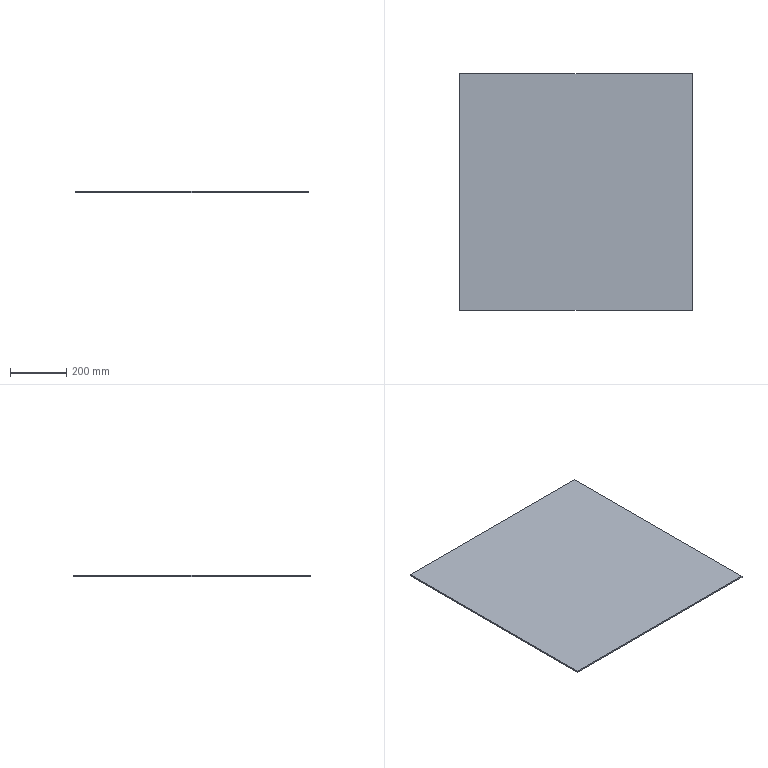Part | SolidWorks | features Extrusion 1, HoleWzd 1 | 1 solid | 6 faces | box 829 x 842 x 5 mm | volume 3490090 mm3 | plane 6
STEP:
#1=CARTESIAN_POINT('',(414.5,-421.,0.));
#2=VERTEX_POINT('',#1);
#3=CARTESIAN_POINT('',(414.5,421.,0.));
#4=VERTEX_POINT('',#3);
#5=CARTESIAN_POINT('',(414.5,421.,0.));
#6=DIRECTION('',(0.,1.,0.));
#7=VECTOR('',#6,1000.);
#8=LINE('',#5,#7);
#9=EDGE_CURVE('',#2,#4,#8,.T.);
#10=ORIENTED_EDGE('',*,*,#9,.T.);
#11=CARTESIAN_POINT('',(414.5,421.,5.));
#12=VERTEX_POINT('',#11);
#13=CARTESIAN_POINT('',(414.5,421.,5.));
#14=DIRECTION('',(0.,0.,-1.));
#15=VECTOR('',#14,1000.);
#16=LINE('',#13,#15);
#17=EDGE_CURVE('',#12,#4,#16,.T.);
#18=ORIENTED_EDGE('',*,*,#17,.F.);
#19=CARTESIAN_POINT('',(414.5,-421.,5.));
#20=VERTEX_POINT('',#19);
#21=CARTESIAN_POINT('',(414.5,421.,5.));
#22=DIRECTION('',(0.,1.,0.));
#23=VECTOR('',#22,1000.);
#24=LINE('',#21,#23);
#25=EDGE_CURVE('',#20,#12,#24,.T.);
#26=ORIENTED_EDGE('',*,*,#25,.F.);
#27=CARTESIAN_POINT('',(414.5,-421.,5.));
#28=DIRECTION('',(0.,0.,-1.));
#29=VECTOR('',#28,1000.);
#30=LINE('',#27,#29);
#31=EDGE_CURVE('',#20,#2,#30,.T.);
#32=ORIENTED_EDGE('',*,*,#31,.T.);
#33=EDGE_LOOP('',(#10,#18,#26,#32));
#34=FACE_OUTER_BOUND('',#33,.T.);
#35=CARTESIAN_POINT('',(414.5,421.,5.));
#36=DIRECTION('',(-1.,0.,0.));
#37=DIRECTION('',(0.,-1.,0.));
#38=AXIS2_PLACEMENT_3D('',#35,#36,#37);
#39=PLANE('',#38);
#40=ADVANCED_FACE('',(#34),#39,.F.);
#41=CARTESIAN_POINT('',(-414.5,421.,0.));
#42=VERTEX_POINT('',#41);
#43=CARTESIAN_POINT('',(-414.5,421.,0.));
#44=DIRECTION('',(-1.,0.,0.));
#45=VECTOR('',#44,1000.);
#46=LINE('',#43,#45);
#47=EDGE_CURVE('',#4,#42,#46,.T.);
#48=ORIENTED_EDGE('',*,*,#47,.T.);
#49=CARTESIAN_POINT('',(-414.5,421.,5.));
#50=VERTEX_POINT('',#49);
#51=CARTESIAN_POINT('',(-414.5,421.,5.));
#52=DIRECTION('',(0.,0.,-1.));
#53=VECTOR('',#52,1000.);
#54=LINE('',#51,#53);
#55=EDGE_CURVE('',#50,#42,#54,.T.);
#56=ORIENTED_EDGE('',*,*,#55,.F.);
#57=CARTESIAN_POINT('',(-414.5,421.,5.));
#58=DIRECTION('',(-1.,0.,0.));
#59=VECTOR('',#58,1000.);
#60=LINE('',#57,#59);
#61=EDGE_CURVE('',#12,#50,#60,.T.);
#62=ORIENTED_EDGE('',*,*,#61,.F.);
#63=ORIENTED_EDGE('',*,*,#17,.T.);
#64=EDGE_LOOP('',(#48,#56,#62,#63));
#65=FACE_OUTER_BOUND('',#64,.T.);
#66=CARTESIAN_POINT('',(-414.5,421.,5.));
#67=DIRECTION('',(0.,-1.,0.));
#68=DIRECTION('',(0.,0.,-1.));
#69=AXIS2_PLACEMENT_3D('',#66,#67,#68);
#70=PLANE('',#69);
#71=ADVANCED_FACE('',(#65),#70,.F.);
#72=CARTESIAN_POINT('',(-414.5,-421.,0.));
#73=VERTEX_POINT('',#72);
#74=CARTESIAN_POINT('',(-414.5,421.,0.));
#75=DIRECTION('',(0.,-1.,0.));
#76=VECTOR('',#75,1000.);
#77=LINE('',#74,#76);
#78=EDGE_CURVE('',#42,#73,#77,.T.);
#79=ORIENTED_EDGE('',*,*,#78,.T.);
#80=CARTESIAN_POINT('',(-414.5,-421.,5.));
#81=VERTEX_POINT('',#80);
#82=CARTESIAN_POINT('',(-414.5,-421.,5.));
#83=DIRECTION('',(0.,0.,-1.));
#84=VECTOR('',#83,1000.);
#85=LINE('',#82,#84);
#86=EDGE_CURVE('',#81,#73,#85,.T.);
#87=ORIENTED_EDGE('',*,*,#86,.F.);
#88=CARTESIAN_POINT('',(-414.5,421.,5.));
#89=DIRECTION('',(0.,-1.,0.));
#90=VECTOR('',#89,1000.);
#91=LINE('',#88,#90);
#92=EDGE_CURVE('',#50,#81,#91,.T.);
#93=ORIENTED_EDGE('',*,*,#92,.F.);
#94=ORIENTED_EDGE('',*,*,#55,.T.);
#95=EDGE_LOOP('',(#79,#87,#93,#94));
#96=FACE_OUTER_BOUND('',#95,.T.);
#97=CARTESIAN_POINT('',(-414.5,421.,5.));
#98=DIRECTION('',(1.,0.,0.));
#99=DIRECTION('',(0.,1.,0.));
#100=AXIS2_PLACEMENT_3D('',#97,#98,#99);
#101=PLANE('',#100);
#102=ADVANCED_FACE('',(#96),#101,.F.);
#103=CARTESIAN_POINT('',(-414.5,-421.,0.));
#104=DIRECTION('',(1.,0.,0.));
#105=VECTOR('',#104,1000.);
#106=LINE('',#103,#105);
#107=EDGE_CURVE('',#73,#2,#106,.T.);
#108=ORIENTED_EDGE('',*,*,#107,.T.);
#109=ORIENTED_EDGE('',*,*,#31,.F.);
#110=CARTESIAN_POINT('',(-414.5,-421.,5.));
#111=DIRECTION('',(1.,0.,0.));
#112=VECTOR('',#111,1000.);
#113=LINE('',#110,#112);
#114=EDGE_CURVE('',#81,#20,#113,.T.);
#115=ORIENTED_EDGE('',*,*,#114,.F.);
#116=ORIENTED_EDGE('',*,*,#86,.T.);
#117=EDGE_LOOP('',(#108,#109,#115,#116));
#118=FACE_OUTER_BOUND('',#117,.T.);
#119=CARTESIAN_POINT('',(-414.5,-421.,5.));
#120=DIRECTION('',(0.,1.,0.));
#121=DIRECTION('',(0.,0.,1.));
#122=AXIS2_PLACEMENT_3D('',#119,#120,#121);
#123=PLANE('',#122);
#124=ADVANCED_FACE('',(#118),#123,.F.);
#125=ORIENTED_EDGE('',*,*,#25,.T.);
#126=ORIENTED_EDGE('',*,*,#61,.T.);
#127=ORIENTED_EDGE('',*,*,#92,.T.);
#128=ORIENTED_EDGE('',*,*,#114,.T.);
#129=EDGE_LOOP('',(#125,#126,#127,#128));
#130=FACE_OUTER_BOUND('',#129,.T.);
#131=CARTESIAN_POINT('',(0.,0.,5.));
#132=DIRECTION('',(0.,0.,1.));
#133=DIRECTION('',(1.,0.,0.));
#134=AXIS2_PLACEMENT_3D('',#131,#132,#133);
#135=PLANE('',#134);
#136=ADVANCED_FACE('',(#130),#135,.T.);
#137=ORIENTED_EDGE('',*,*,#9,.F.);
#138=ORIENTED_EDGE('',*,*,#107,.F.);
#139=ORIENTED_EDGE('',*,*,#78,.F.);
#140=ORIENTED_EDGE('',*,*,#47,.F.);
#141=EDGE_LOOP('',(#137,#138,#139,#140));
#142=FACE_OUTER_BOUND('',#141,.T.);
#143=CARTESIAN_POINT('',(0.,0.,0.));
#144=DIRECTION('',(0.,0.,1.));
#145=DIRECTION('',(1.,0.,0.));
#146=AXIS2_PLACEMENT_3D('',#143,#144,#145);
#147=PLANE('',#146);
#148=ADVANCED_FACE('',(#142),#147,.F.);
#149=CLOSED_SHELL('',(#40,#71,#102,#124,#136,#148));
#150=MANIFOLD_SOLID_BREP('',#149);
#151=CARTESIAN_POINT('',(0.,0.,0.));
#152=DIRECTION('',(0.,0.,1.));
#153=DIRECTION('',(1.,0.,0.));
#154=AXIS2_PLACEMENT_3D('',#151,#152,#153);
#155=(LENGTH_UNIT()NAMED_UNIT(*)SI_UNIT(.MILLI.,.METRE.));
#156=UNCERTAINTY_MEASURE_WITH_UNIT(LENGTH_MEASURE(0.00001),#155,'','');
#157=(NAMED_UNIT(*)PLANE_ANGLE_UNIT()SI_UNIT($,.RADIAN.));
#158=(NAMED_UNIT(*)SI_UNIT($,.STERADIAN.)SOLID_ANGLE_UNIT());
#159=(GEOMETRIC_REPRESENTATION_CONTEXT(3)GLOBAL_UNCERTAINTY_ASSIGNED_CONTEXT((#156))GLOBAL_UNIT_ASSIGNED_CONTEXT((#155,#157,#158))REPRESENTATION_CONTEXT('',''));
#160=ADVANCED_BREP_SHAPE_REPRESENTATION('',(#150,#154),#159);